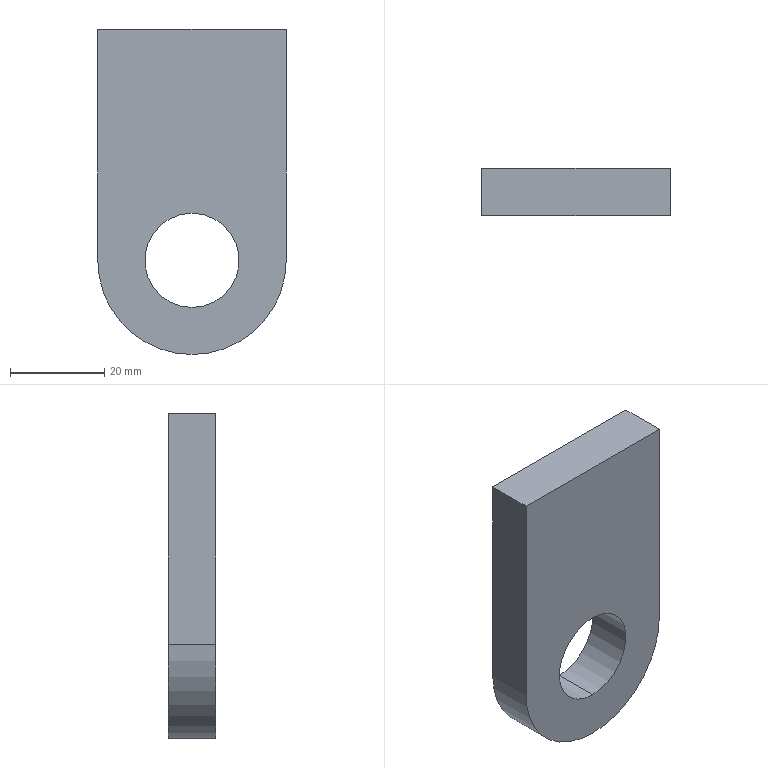Part | SolidWorks | features Extrusion 1 | 1 solid | 9 faces | box 40 x 10 x 69.01 mm | volume 22746 mm3 | plane 5 | cylinder 4 | commonest cylinder face diameters 20 x2 40 x2
STEP:
#1=CARTESIAN_POINT('',(0.,5.,-34.505));
#2=VERTEX_POINT('',#1);
#3=CARTESIAN_POINT('',(0.,5.,-14.505));
#4=VERTEX_POINT('',#3);
#5=CARTESIAN_POINT('',(0.,5.,-24.505));
#6=DIRECTION('',(0.,1.,0.));
#7=DIRECTION('',(0.,0.,1.));
#8=AXIS2_PLACEMENT_3D('',#5,#6,#7);
#9=CIRCLE('',#8,10.);
#10=EDGE_CURVE('',#2,#4,#9,.T.);
#11=ORIENTED_EDGE('',*,*,#10,.T.);
#12=CARTESIAN_POINT('',(0.,-5.,-14.505));
#13=VERTEX_POINT('',#12);
#14=CARTESIAN_POINT('',(0.,5.,-14.505));
#15=DIRECTION('',(0.,-1.,0.));
#16=VECTOR('',#15,1000.);
#17=LINE('',#14,#16);
#18=EDGE_CURVE('',#4,#13,#17,.T.);
#19=ORIENTED_EDGE('',*,*,#18,.T.);
#20=CARTESIAN_POINT('',(0.,-5.,-34.505));
#21=VERTEX_POINT('',#20);
#22=CARTESIAN_POINT('',(0.,-5.,-24.505));
#23=DIRECTION('',(0.,1.,0.));
#24=DIRECTION('',(0.,0.,1.));
#25=AXIS2_PLACEMENT_3D('',#22,#23,#24);
#26=CIRCLE('',#25,10.);
#27=EDGE_CURVE('',#21,#13,#26,.T.);
#28=ORIENTED_EDGE('',*,*,#27,.F.);
#29=CARTESIAN_POINT('',(0.,5.,-34.505));
#30=DIRECTION('',(0.,-1.,0.));
#31=VECTOR('',#30,1000.);
#32=LINE('',#29,#31);
#33=EDGE_CURVE('',#2,#21,#32,.T.);
#34=ORIENTED_EDGE('',*,*,#33,.F.);
#35=EDGE_LOOP('',(#11,#19,#28,#34));
#36=FACE_OUTER_BOUND('',#35,.T.);
#37=CARTESIAN_POINT('',(0.,5.,-24.505));
#38=DIRECTION('',(0.,-1.,0.));
#39=DIRECTION('',(0.,0.,-1.));
#40=AXIS2_PLACEMENT_3D('',#37,#38,#39);
#41=CYLINDRICAL_SURFACE('',#40,10.);
#42=ADVANCED_FACE('',(#36),#41,.F.);
#43=CARTESIAN_POINT('',(0.,5.,-44.505));
#44=VERTEX_POINT('',#43);
#45=CARTESIAN_POINT('',(-20.,5.,-24.505));
#46=VERTEX_POINT('',#45);
#47=CARTESIAN_POINT('',(0.,5.,-24.505));
#48=DIRECTION('',(0.,1.,0.));
#49=DIRECTION('',(0.,0.,1.));
#50=AXIS2_PLACEMENT_3D('',#47,#48,#49);
#51=CIRCLE('',#50,20.);
#52=EDGE_CURVE('',#44,#46,#51,.T.);
#53=ORIENTED_EDGE('',*,*,#52,.F.);
#54=CARTESIAN_POINT('',(0.,-5.,-44.505));
#55=VERTEX_POINT('',#54);
#56=CARTESIAN_POINT('',(0.,5.,-44.505));
#57=DIRECTION('',(0.,-1.,0.));
#58=VECTOR('',#57,1000.);
#59=LINE('',#56,#58);
#60=EDGE_CURVE('',#44,#55,#59,.T.);
#61=ORIENTED_EDGE('',*,*,#60,.T.);
#62=CARTESIAN_POINT('',(-20.,-5.,-24.505));
#63=VERTEX_POINT('',#62);
#64=CARTESIAN_POINT('',(0.,-5.,-24.505));
#65=DIRECTION('',(0.,1.,0.));
#66=DIRECTION('',(0.,0.,1.));
#67=AXIS2_PLACEMENT_3D('',#64,#65,#66);
#68=CIRCLE('',#67,20.);
#69=EDGE_CURVE('',#55,#63,#68,.T.);
#70=ORIENTED_EDGE('',*,*,#69,.T.);
#71=CARTESIAN_POINT('',(-20.,5.,-24.505));
#72=DIRECTION('',(0.,-1.,0.));
#73=VECTOR('',#72,1000.);
#74=LINE('',#71,#73);
#75=EDGE_CURVE('',#46,#63,#74,.T.);
#76=ORIENTED_EDGE('',*,*,#75,.F.);
#77=EDGE_LOOP('',(#53,#61,#70,#76));
#78=FACE_OUTER_BOUND('',#77,.T.);
#79=CARTESIAN_POINT('',(0.,5.,-24.505));
#80=DIRECTION('',(0.,-1.,0.));
#81=DIRECTION('',(0.,0.,-1.));
#82=AXIS2_PLACEMENT_3D('',#79,#80,#81);
#83=CYLINDRICAL_SURFACE('',#82,20.);
#84=ADVANCED_FACE('',(#78),#83,.T.);
#85=CARTESIAN_POINT('',(20.,5.,-24.505));
#86=VERTEX_POINT('',#85);
#87=CARTESIAN_POINT('',(0.,5.,-24.505));
#88=DIRECTION('',(0.,1.,0.));
#89=DIRECTION('',(0.,0.,1.));
#90=AXIS2_PLACEMENT_3D('',#87,#88,#89);
#91=CIRCLE('',#90,20.);
#92=EDGE_CURVE('',#86,#44,#91,.T.);
#93=ORIENTED_EDGE('',*,*,#92,.T.);
#94=ORIENTED_EDGE('',*,*,#52,.T.);
#95=CARTESIAN_POINT('',(-20.,5.,24.505));
#96=VERTEX_POINT('',#95);
#97=CARTESIAN_POINT('',(-20.,5.,24.505));
#98=DIRECTION('',(0.,0.,1.));
#99=VECTOR('',#98,1000.);
#100=LINE('',#97,#99);
#101=EDGE_CURVE('',#46,#96,#100,.T.);
#102=ORIENTED_EDGE('',*,*,#101,.T.);
#103=CARTESIAN_POINT('',(20.,5.,24.505));
#104=VERTEX_POINT('',#103);
#105=CARTESIAN_POINT('',(-20.,5.,24.505));
#106=DIRECTION('',(1.,0.,0.));
#107=VECTOR('',#106,1000.);
#108=LINE('',#105,#107);
#109=EDGE_CURVE('',#96,#104,#108,.T.);
#110=ORIENTED_EDGE('',*,*,#109,.T.);
#111=CARTESIAN_POINT('',(20.,5.,24.505));
#112=DIRECTION('',(0.,0.,-1.));
#113=VECTOR('',#112,1000.);
#114=LINE('',#111,#113);
#115=EDGE_CURVE('',#104,#86,#114,.T.);
#116=ORIENTED_EDGE('',*,*,#115,.T.);
#117=EDGE_LOOP('',(#93,#94,#102,#110,#116));
#118=FACE_OUTER_BOUND('',#117,.T.);
#119=ORIENTED_EDGE('',*,*,#10,.F.);
#120=CARTESIAN_POINT('',(0.,5.,-24.505));
#121=DIRECTION('',(0.,1.,0.));
#122=DIRECTION('',(0.,0.,1.));
#123=AXIS2_PLACEMENT_3D('',#120,#121,#122);
#124=CIRCLE('',#123,10.);
#125=EDGE_CURVE('',#4,#2,#124,.T.);
#126=ORIENTED_EDGE('',*,*,#125,.F.);
#127=EDGE_LOOP('',(#119,#126));
#128=FACE_BOUND('',#127,.T.);
#129=CARTESIAN_POINT('',(0.,5.,-24.505));
#130=DIRECTION('',(0.,1.,0.));
#131=DIRECTION('',(0.,0.,1.));
#132=AXIS2_PLACEMENT_3D('',#129,#130,#131);
#133=PLANE('',#132);
#134=ADVANCED_FACE('',(#118,#128),#133,.T.);
#135=CARTESIAN_POINT('',(20.,-5.,-24.505));
#136=VERTEX_POINT('',#135);
#137=CARTESIAN_POINT('',(0.,-5.,-24.505));
#138=DIRECTION('',(0.,1.,0.));
#139=DIRECTION('',(0.,0.,1.));
#140=AXIS2_PLACEMENT_3D('',#137,#138,#139);
#141=CIRCLE('',#140,20.);
#142=EDGE_CURVE('',#136,#55,#141,.T.);
#143=ORIENTED_EDGE('',*,*,#142,.F.);
#144=CARTESIAN_POINT('',(20.,-5.,24.505));
#145=VERTEX_POINT('',#144);
#146=CARTESIAN_POINT('',(20.,-5.,24.505));
#147=DIRECTION('',(0.,0.,-1.));
#148=VECTOR('',#147,1000.);
#149=LINE('',#146,#148);
#150=EDGE_CURVE('',#145,#136,#149,.T.);
#151=ORIENTED_EDGE('',*,*,#150,.F.);
#152=CARTESIAN_POINT('',(-20.,-5.,24.505));
#153=VERTEX_POINT('',#152);
#154=CARTESIAN_POINT('',(-20.,-5.,24.505));
#155=DIRECTION('',(1.,0.,0.));
#156=VECTOR('',#155,1000.);
#157=LINE('',#154,#156);
#158=EDGE_CURVE('',#153,#145,#157,.T.);
#159=ORIENTED_EDGE('',*,*,#158,.F.);
#160=CARTESIAN_POINT('',(-20.,-5.,24.505));
#161=DIRECTION('',(0.,0.,1.));
#162=VECTOR('',#161,1000.);
#163=LINE('',#160,#162);
#164=EDGE_CURVE('',#63,#153,#163,.T.);
#165=ORIENTED_EDGE('',*,*,#164,.F.);
#166=ORIENTED_EDGE('',*,*,#69,.F.);
#167=EDGE_LOOP('',(#143,#151,#159,#165,#166));
#168=FACE_OUTER_BOUND('',#167,.T.);
#169=ORIENTED_EDGE('',*,*,#27,.T.);
#170=CARTESIAN_POINT('',(0.,-5.,-24.505));
#171=DIRECTION('',(0.,1.,0.));
#172=DIRECTION('',(0.,0.,1.));
#173=AXIS2_PLACEMENT_3D('',#170,#171,#172);
#174=CIRCLE('',#173,10.);
#175=EDGE_CURVE('',#13,#21,#174,.T.);
#176=ORIENTED_EDGE('',*,*,#175,.T.);
#177=EDGE_LOOP('',(#169,#176));
#178=FACE_BOUND('',#177,.T.);
#179=CARTESIAN_POINT('',(0.,-5.,-24.505));
#180=DIRECTION('',(0.,1.,0.));
#181=DIRECTION('',(0.,0.,1.));
#182=AXIS2_PLACEMENT_3D('',#179,#180,#181);
#183=PLANE('',#182);
#184=ADVANCED_FACE('',(#168,#178),#183,.F.);
#185=ORIENTED_EDGE('',*,*,#60,.F.);
#186=ORIENTED_EDGE('',*,*,#92,.F.);
#187=CARTESIAN_POINT('',(20.,5.,-24.505));
#188=DIRECTION('',(0.,-1.,0.));
#189=VECTOR('',#188,1000.);
#190=LINE('',#187,#189);
#191=EDGE_CURVE('',#86,#136,#190,.T.);
#192=ORIENTED_EDGE('',*,*,#191,.T.);
#193=ORIENTED_EDGE('',*,*,#142,.T.);
#194=EDGE_LOOP('',(#185,#186,#192,#193));
#195=FACE_OUTER_BOUND('',#194,.T.);
#196=CARTESIAN_POINT('',(0.,5.,-24.505));
#197=DIRECTION('',(0.,-1.,0.));
#198=DIRECTION('',(0.,0.,-1.));
#199=AXIS2_PLACEMENT_3D('',#196,#197,#198);
#200=CYLINDRICAL_SURFACE('',#199,20.);
#201=ADVANCED_FACE('',(#195),#200,.T.);
#202=ORIENTED_EDGE('',*,*,#164,.T.);
#203=CARTESIAN_POINT('',(-20.,5.,24.505));
#204=DIRECTION('',(0.,-1.,0.));
#205=VECTOR('',#204,1000.);
#206=LINE('',#203,#205);
#207=EDGE_CURVE('',#96,#153,#206,.T.);
#208=ORIENTED_EDGE('',*,*,#207,.F.);
#209=ORIENTED_EDGE('',*,*,#101,.F.);
#210=ORIENTED_EDGE('',*,*,#75,.T.);
#211=EDGE_LOOP('',(#202,#208,#209,#210));
#212=FACE_OUTER_BOUND('',#211,.T.);
#213=CARTESIAN_POINT('',(-20.,5.,24.505));
#214=DIRECTION('',(1.,0.,0.));
#215=DIRECTION('',(0.,0.,-1.));
#216=AXIS2_PLACEMENT_3D('',#213,#214,#215);
#217=PLANE('',#216);
#218=ADVANCED_FACE('',(#212),#217,.F.);
#219=ORIENTED_EDGE('',*,*,#158,.T.);
#220=CARTESIAN_POINT('',(20.,5.,24.505));
#221=DIRECTION('',(0.,-1.,0.));
#222=VECTOR('',#221,1000.);
#223=LINE('',#220,#222);
#224=EDGE_CURVE('',#104,#145,#223,.T.);
#225=ORIENTED_EDGE('',*,*,#224,.F.);
#226=ORIENTED_EDGE('',*,*,#109,.F.);
#227=ORIENTED_EDGE('',*,*,#207,.T.);
#228=EDGE_LOOP('',(#219,#225,#226,#227));
#229=FACE_OUTER_BOUND('',#228,.T.);
#230=CARTESIAN_POINT('',(-20.,5.,24.505));
#231=DIRECTION('',(0.,0.,-1.));
#232=DIRECTION('',(-1.,0.,0.));
#233=AXIS2_PLACEMENT_3D('',#230,#231,#232);
#234=PLANE('',#233);
#235=ADVANCED_FACE('',(#229),#234,.F.);
#236=ORIENTED_EDGE('',*,*,#150,.T.);
#237=ORIENTED_EDGE('',*,*,#191,.F.);
#238=ORIENTED_EDGE('',*,*,#115,.F.);
#239=ORIENTED_EDGE('',*,*,#224,.T.);
#240=EDGE_LOOP('',(#236,#237,#238,#239));
#241=FACE_OUTER_BOUND('',#240,.T.);
#242=CARTESIAN_POINT('',(20.,5.,24.505));
#243=DIRECTION('',(-1.,0.,0.));
#244=DIRECTION('',(0.,0.,1.));
#245=AXIS2_PLACEMENT_3D('',#242,#243,#244);
#246=PLANE('',#245);
#247=ADVANCED_FACE('',(#241),#246,.F.);
#248=ORIENTED_EDGE('',*,*,#18,.F.);
#249=ORIENTED_EDGE('',*,*,#125,.T.);
#250=ORIENTED_EDGE('',*,*,#33,.T.);
#251=ORIENTED_EDGE('',*,*,#175,.F.);
#252=EDGE_LOOP('',(#248,#249,#250,#251));
#253=FACE_OUTER_BOUND('',#252,.T.);
#254=CARTESIAN_POINT('',(0.,5.,-24.505));
#255=DIRECTION('',(0.,-1.,0.));
#256=DIRECTION('',(0.,0.,-1.));
#257=AXIS2_PLACEMENT_3D('',#254,#255,#256);
#258=CYLINDRICAL_SURFACE('',#257,10.);
#259=ADVANCED_FACE('',(#253),#258,.F.);
#260=CLOSED_SHELL('',(#42,#84,#134,#184,#201,#218,#235,#247,#259));
#261=MANIFOLD_SOLID_BREP('',#260);
#262=CARTESIAN_POINT('',(0.,0.,0.));
#263=DIRECTION('',(0.,0.,1.));
#264=DIRECTION('',(1.,0.,0.));
#265=AXIS2_PLACEMENT_3D('',#262,#263,#264);
#266=(LENGTH_UNIT()NAMED_UNIT(*)SI_UNIT(.MILLI.,.METRE.));
#267=UNCERTAINTY_MEASURE_WITH_UNIT(LENGTH_MEASURE(0.00001),#266,'','');
#268=(NAMED_UNIT(*)PLANE_ANGLE_UNIT()SI_UNIT($,.RADIAN.));
#269=(NAMED_UNIT(*)SI_UNIT($,.STERADIAN.)SOLID_ANGLE_UNIT());
#270=(GEOMETRIC_REPRESENTATION_CONTEXT(3)GLOBAL_UNCERTAINTY_ASSIGNED_CONTEXT((#267))GLOBAL_UNIT_ASSIGNED_CONTEXT((#266,#268,#269))REPRESENTATION_CONTEXT('',''));
#271=ADVANCED_BREP_SHAPE_REPRESENTATION('',(#261,#265),#270);